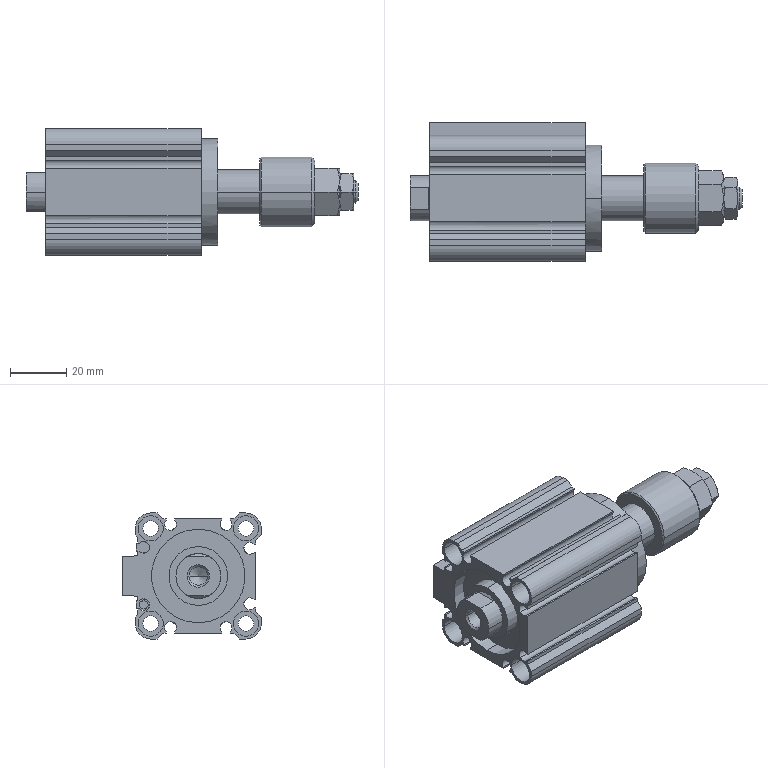Part | STEP file | CDQ2B32-15DZ-M9NL-XC8_0_XC8_0_^Cylinder clamp assembly | 5 solids | 284 faces | box 118.5 x 49.5 x 45 mm | volume 100397 mm3 | plane 140 | cylinder 102 | cone 40 | torus 2 | commonest cylinder face diameters 4.26 x16 9 x16 0.6 x8 5.5 x8 16 x8 2 x4